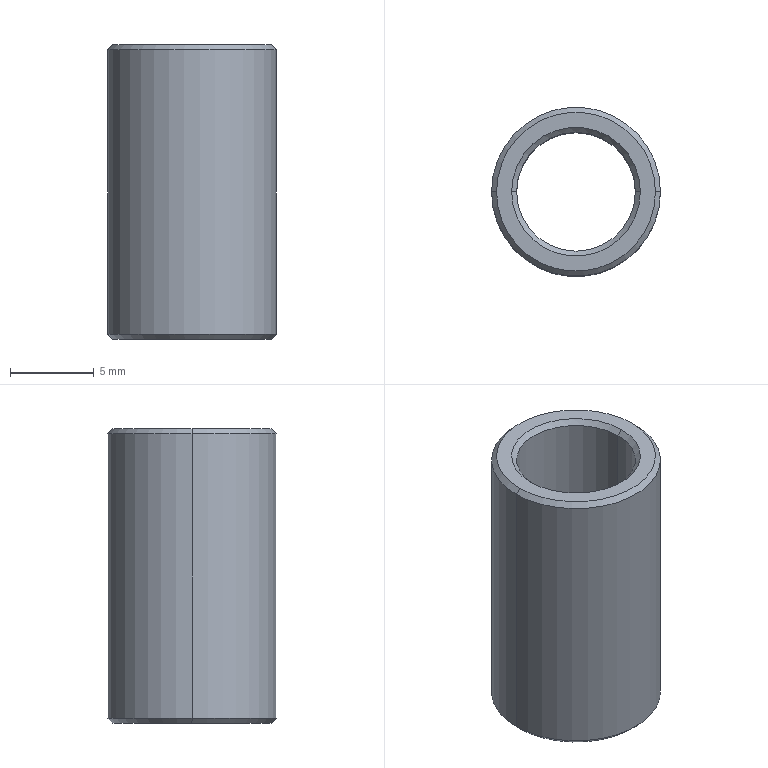Part | NX | features BREP 1 | 1 solid | 14 faces | box 10.1 x 10.1 x 17.6 mm | volume 708.404 mm3 | cone 8 | cylinder 4 | plane 2 | commonest cylinder face diameters 7.1 x2 10.1 x2
STEP:
#1=CARTESIAN_POINT('',(-5.05,0.,0.3));
#2=VERTEX_POINT('',#1);
#3=CARTESIAN_POINT('',(-4.75,0.,0.));
#4=VERTEX_POINT('',#3);
#5=CARTESIAN_POINT('',(-5.05,0.,0.3));
#6=DIRECTION('',(-0.7071,0.,0.7071));
#7=VECTOR('',#6,1000.);
#8=LINE('',#5,#7);
#9=EDGE_CURVE('',#2,#4,#8,.F.);
#10=ORIENTED_EDGE('',*,*,#9,.T.);
#11=CARTESIAN_POINT('',(4.75,0.,0.));
#12=VERTEX_POINT('',#11);
#13=CARTESIAN_POINT('',(0.,0.,0.));
#14=DIRECTION('',(0.,0.,-1.));
#15=DIRECTION('',(1.,0.,0.));
#16=AXIS2_PLACEMENT_3D('',#13,#14,#15);
#17=CIRCLE('',#16,4.75);
#18=EDGE_CURVE('',#12,#4,#17,.T.);
#19=ORIENTED_EDGE('',*,*,#18,.F.);
#20=CARTESIAN_POINT('',(5.05,0.,0.3));
#21=VERTEX_POINT('',#20);
#22=CARTESIAN_POINT('',(5.05,0.,0.3));
#23=DIRECTION('',(0.7071,0.,0.7071));
#24=VECTOR('',#23,1000.);
#25=LINE('',#22,#24);
#26=EDGE_CURVE('',#21,#12,#25,.F.);
#27=ORIENTED_EDGE('',*,*,#26,.F.);
#28=CARTESIAN_POINT('',(0.,0.,0.3));
#29=DIRECTION('',(0.,0.,1.));
#30=DIRECTION('',(1.,0.,0.));
#31=AXIS2_PLACEMENT_3D('',#28,#29,#30);
#32=CIRCLE('',#31,5.05);
#33=EDGE_CURVE('',#2,#21,#32,.T.);
#34=ORIENTED_EDGE('',*,*,#33,.F.);
#35=EDGE_LOOP('',(#10,#19,#27,#34));
#36=FACE_BOUND('',#35,.T.);
#37=CARTESIAN_POINT('',(0.,0.,0.3));
#38=DIRECTION('',(0.,0.,1.));
#39=DIRECTION('',(1.,0.,0.));
#40=AXIS2_PLACEMENT_3D('',#37,#38,#39);
#41=CONICAL_SURFACE('',#40,5.05,0.7854);
#42=ADVANCED_FACE('',(#36),#41,.T.);
#43=CARTESIAN_POINT('',(3.55,0.,0.3));
#44=VERTEX_POINT('',#43);
#45=CARTESIAN_POINT('',(3.85,0.,0.));
#46=VERTEX_POINT('',#45);
#47=CARTESIAN_POINT('',(3.85,0.,0.));
#48=DIRECTION('',(0.7071,0.,-0.7071));
#49=VECTOR('',#48,1000.);
#50=LINE('',#47,#49);
#51=EDGE_CURVE('',#44,#46,#50,.T.);
#52=ORIENTED_EDGE('',*,*,#51,.F.);
#53=CARTESIAN_POINT('',(-3.55,0.,0.3));
#54=VERTEX_POINT('',#53);
#55=CARTESIAN_POINT('',(0.,0.,0.3));
#56=DIRECTION('',(0.,0.,-1.));
#57=DIRECTION('',(1.,0.,0.));
#58=AXIS2_PLACEMENT_3D('',#55,#56,#57);
#59=CIRCLE('',#58,3.55);
#60=EDGE_CURVE('',#54,#44,#59,.T.);
#61=ORIENTED_EDGE('',*,*,#60,.F.);
#62=CARTESIAN_POINT('',(-3.85,0.,0.));
#63=VERTEX_POINT('',#62);
#64=CARTESIAN_POINT('',(-3.85,0.,0.));
#65=DIRECTION('',(-0.7071,0.,-0.7071));
#66=VECTOR('',#65,1000.);
#67=LINE('',#64,#66);
#68=EDGE_CURVE('',#54,#63,#67,.T.);
#69=ORIENTED_EDGE('',*,*,#68,.T.);
#70=CARTESIAN_POINT('',(0.,0.,0.));
#71=DIRECTION('',(0.,0.,1.));
#72=DIRECTION('',(1.,0.,0.));
#73=AXIS2_PLACEMENT_3D('',#70,#71,#72);
#74=CIRCLE('',#73,3.85);
#75=EDGE_CURVE('',#46,#63,#74,.T.);
#76=ORIENTED_EDGE('',*,*,#75,.F.);
#77=EDGE_LOOP('',(#52,#61,#69,#76));
#78=FACE_BOUND('',#77,.T.);
#79=CARTESIAN_POINT('',(0.,0.,0.));
#80=DIRECTION('',(0.,0.,-1.));
#81=DIRECTION('',(-1.,0.,0.));
#82=AXIS2_PLACEMENT_3D('',#79,#80,#81);
#83=CONICAL_SURFACE('',#82,3.85,0.7854);
#84=ADVANCED_FACE('',(#78),#83,.F.);
#85=CARTESIAN_POINT('',(4.75,0.,17.6));
#86=VERTEX_POINT('',#85);
#87=CARTESIAN_POINT('',(5.05,0.,17.3));
#88=VERTEX_POINT('',#87);
#89=CARTESIAN_POINT('',(4.75,0.,17.6));
#90=DIRECTION('',(0.7071,0.,-0.7071));
#91=VECTOR('',#90,1000.);
#92=LINE('',#89,#91);
#93=EDGE_CURVE('',#86,#88,#92,.T.);
#94=ORIENTED_EDGE('',*,*,#93,.F.);
#95=CARTESIAN_POINT('',(-4.75,0.,17.6));
#96=VERTEX_POINT('',#95);
#97=CARTESIAN_POINT('',(0.,0.,17.6));
#98=DIRECTION('',(0.,0.,1.));
#99=DIRECTION('',(1.,0.,0.));
#100=AXIS2_PLACEMENT_3D('',#97,#98,#99);
#101=CIRCLE('',#100,4.75);
#102=EDGE_CURVE('',#96,#86,#101,.T.);
#103=ORIENTED_EDGE('',*,*,#102,.F.);
#104=CARTESIAN_POINT('',(-5.05,0.,17.3));
#105=VERTEX_POINT('',#104);
#106=CARTESIAN_POINT('',(-4.75,0.,17.6));
#107=DIRECTION('',(-0.7071,0.,-0.7071));
#108=VECTOR('',#107,1000.);
#109=LINE('',#106,#108);
#110=EDGE_CURVE('',#96,#105,#109,.T.);
#111=ORIENTED_EDGE('',*,*,#110,.T.);
#112=CARTESIAN_POINT('',(0.,0.,17.3));
#113=DIRECTION('',(0.,0.,-1.));
#114=DIRECTION('',(1.,0.,0.));
#115=AXIS2_PLACEMENT_3D('',#112,#113,#114);
#116=CIRCLE('',#115,5.05);
#117=EDGE_CURVE('',#88,#105,#116,.T.);
#118=ORIENTED_EDGE('',*,*,#117,.F.);
#119=EDGE_LOOP('',(#94,#103,#111,#118));
#120=FACE_BOUND('',#119,.T.);
#121=CARTESIAN_POINT('',(0.,0.,17.6));
#122=DIRECTION('',(0.,0.,-1.));
#123=DIRECTION('',(-1.,0.,0.));
#124=AXIS2_PLACEMENT_3D('',#121,#122,#123);
#125=CONICAL_SURFACE('',#124,4.75,0.7854);
#126=ADVANCED_FACE('',(#120),#125,.T.);
#127=CARTESIAN_POINT('',(-3.85,0.,17.6));
#128=VERTEX_POINT('',#127);
#129=CARTESIAN_POINT('',(-3.55,0.,17.3));
#130=VERTEX_POINT('',#129);
#131=CARTESIAN_POINT('',(-3.55,0.,17.3));
#132=DIRECTION('',(-0.7071,0.,0.7071));
#133=VECTOR('',#132,1000.);
#134=LINE('',#131,#133);
#135=EDGE_CURVE('',#128,#130,#134,.F.);
#136=ORIENTED_EDGE('',*,*,#135,.T.);
#137=CARTESIAN_POINT('',(3.55,0.,17.3));
#138=VERTEX_POINT('',#137);
#139=CARTESIAN_POINT('',(0.,0.,17.3));
#140=DIRECTION('',(0.,0.,1.));
#141=DIRECTION('',(1.,0.,0.));
#142=AXIS2_PLACEMENT_3D('',#139,#140,#141);
#143=CIRCLE('',#142,3.55);
#144=EDGE_CURVE('',#138,#130,#143,.T.);
#145=ORIENTED_EDGE('',*,*,#144,.F.);
#146=CARTESIAN_POINT('',(3.85,0.,17.6));
#147=VERTEX_POINT('',#146);
#148=CARTESIAN_POINT('',(3.55,0.,17.3));
#149=DIRECTION('',(0.7071,0.,0.7071));
#150=VECTOR('',#149,1000.);
#151=LINE('',#148,#150);
#152=EDGE_CURVE('',#147,#138,#151,.F.);
#153=ORIENTED_EDGE('',*,*,#152,.F.);
#154=CARTESIAN_POINT('',(0.,0.,17.6));
#155=DIRECTION('',(0.,0.,-1.));
#156=DIRECTION('',(1.,0.,0.));
#157=AXIS2_PLACEMENT_3D('',#154,#155,#156);
#158=CIRCLE('',#157,3.85);
#159=EDGE_CURVE('',#128,#147,#158,.T.);
#160=ORIENTED_EDGE('',*,*,#159,.F.);
#161=EDGE_LOOP('',(#136,#145,#153,#160));
#162=FACE_BOUND('',#161,.T.);
#163=CARTESIAN_POINT('',(0.,0.,17.3));
#164=DIRECTION('',(0.,0.,1.));
#165=DIRECTION('',(1.,0.,0.));
#166=AXIS2_PLACEMENT_3D('',#163,#164,#165);
#167=CONICAL_SURFACE('',#166,3.55,0.7854);
#168=ADVANCED_FACE('',(#162),#167,.F.);
#169=CARTESIAN_POINT('',(3.55,0.,17.6));
#170=DIRECTION('',(0.,0.,-1.));
#171=VECTOR('',#170,1000.);
#172=LINE('',#169,#171);
#173=EDGE_CURVE('',#138,#44,#172,.T.);
#174=ORIENTED_EDGE('',*,*,#173,.F.);
#175=ORIENTED_EDGE('',*,*,#144,.T.);
#176=CARTESIAN_POINT('',(-3.55,0.,17.6));
#177=DIRECTION('',(0.,0.,-1.));
#178=VECTOR('',#177,1000.);
#179=LINE('',#176,#178);
#180=EDGE_CURVE('',#130,#54,#179,.T.);
#181=ORIENTED_EDGE('',*,*,#180,.T.);
#182=ORIENTED_EDGE('',*,*,#60,.T.);
#183=EDGE_LOOP('',(#174,#175,#181,#182));
#184=FACE_BOUND('',#183,.T.);
#185=CARTESIAN_POINT('',(0.,0.,17.6));
#186=DIRECTION('',(0.,0.,-1.));
#187=DIRECTION('',(-1.,0.,0.));
#188=AXIS2_PLACEMENT_3D('',#185,#186,#187);
#189=CYLINDRICAL_SURFACE('',#188,3.55);
#190=ADVANCED_FACE('',(#184),#189,.F.);
#191=CARTESIAN_POINT('',(5.05,0.,17.6));
#192=DIRECTION('',(0.,0.,-1.));
#193=VECTOR('',#192,1000.);
#194=LINE('',#191,#193);
#195=EDGE_CURVE('',#88,#21,#194,.T.);
#196=ORIENTED_EDGE('',*,*,#195,.F.);
#197=ORIENTED_EDGE('',*,*,#117,.T.);
#198=CARTESIAN_POINT('',(-5.05,0.,17.6));
#199=DIRECTION('',(0.,0.,-1.));
#200=VECTOR('',#199,1000.);
#201=LINE('',#198,#200);
#202=EDGE_CURVE('',#105,#2,#201,.T.);
#203=ORIENTED_EDGE('',*,*,#202,.T.);
#204=ORIENTED_EDGE('',*,*,#33,.T.);
#205=EDGE_LOOP('',(#196,#197,#203,#204));
#206=FACE_BOUND('',#205,.T.);
#207=CARTESIAN_POINT('',(0.,0.,17.6));
#208=DIRECTION('',(0.,0.,-1.));
#209=DIRECTION('',(-1.,0.,0.));
#210=AXIS2_PLACEMENT_3D('',#207,#208,#209);
#211=CYLINDRICAL_SURFACE('',#210,5.05);
#212=ADVANCED_FACE('',(#206),#211,.T.);
#213=ORIENTED_EDGE('',*,*,#18,.T.);
#214=CARTESIAN_POINT('',(0.,0.,0.));
#215=DIRECTION('',(0.,0.,-1.));
#216=DIRECTION('',(1.,0.,0.));
#217=AXIS2_PLACEMENT_3D('',#214,#215,#216);
#218=CIRCLE('',#217,4.75);
#219=EDGE_CURVE('',#4,#12,#218,.T.);
#220=ORIENTED_EDGE('',*,*,#219,.T.);
#221=EDGE_LOOP('',(#213,#220));
#222=FACE_BOUND('',#221,.T.);
#223=CARTESIAN_POINT('',(0.,0.,0.));
#224=DIRECTION('',(0.,0.,1.));
#225=DIRECTION('',(1.,0.,0.));
#226=AXIS2_PLACEMENT_3D('',#223,#224,#225);
#227=CIRCLE('',#226,3.85);
#228=EDGE_CURVE('',#63,#46,#227,.T.);
#229=ORIENTED_EDGE('',*,*,#228,.T.);
#230=ORIENTED_EDGE('',*,*,#75,.T.);
#231=EDGE_LOOP('',(#229,#230));
#232=FACE_BOUND('',#231,.T.);
#233=CARTESIAN_POINT('',(0.,0.,0.));
#234=DIRECTION('',(0.,0.,1.));
#235=DIRECTION('',(1.,0.,0.));
#236=AXIS2_PLACEMENT_3D('',#233,#234,#235);
#237=PLANE('',#236);
#238=ADVANCED_FACE('',(#222,#232),#237,.F.);
#239=ORIENTED_EDGE('',*,*,#102,.T.);
#240=CARTESIAN_POINT('',(0.,0.,17.6));
#241=DIRECTION('',(0.,0.,1.));
#242=DIRECTION('',(1.,0.,0.));
#243=AXIS2_PLACEMENT_3D('',#240,#241,#242);
#244=CIRCLE('',#243,4.75);
#245=EDGE_CURVE('',#86,#96,#244,.T.);
#246=ORIENTED_EDGE('',*,*,#245,.T.);
#247=EDGE_LOOP('',(#239,#246));
#248=FACE_BOUND('',#247,.T.);
#249=CARTESIAN_POINT('',(0.,0.,17.6));
#250=DIRECTION('',(0.,0.,-1.));
#251=DIRECTION('',(1.,0.,0.));
#252=AXIS2_PLACEMENT_3D('',#249,#250,#251);
#253=CIRCLE('',#252,3.85);
#254=EDGE_CURVE('',#147,#128,#253,.T.);
#255=ORIENTED_EDGE('',*,*,#254,.T.);
#256=ORIENTED_EDGE('',*,*,#159,.T.);
#257=EDGE_LOOP('',(#255,#256));
#258=FACE_BOUND('',#257,.T.);
#259=CARTESIAN_POINT('',(0.,0.,17.6));
#260=DIRECTION('',(0.,0.,1.));
#261=DIRECTION('',(1.,0.,0.));
#262=AXIS2_PLACEMENT_3D('',#259,#260,#261);
#263=PLANE('',#262);
#264=ADVANCED_FACE('',(#248,#258),#263,.T.);
#265=CARTESIAN_POINT('',(0.,0.,17.3));
#266=DIRECTION('',(0.,0.,-1.));
#267=DIRECTION('',(1.,0.,0.));
#268=AXIS2_PLACEMENT_3D('',#265,#266,#267);
#269=CIRCLE('',#268,5.05);
#270=EDGE_CURVE('',#105,#88,#269,.T.);
#271=ORIENTED_EDGE('',*,*,#270,.T.);
#272=ORIENTED_EDGE('',*,*,#195,.T.);
#273=CARTESIAN_POINT('',(0.,0.,0.3));
#274=DIRECTION('',(0.,0.,1.));
#275=DIRECTION('',(1.,0.,0.));
#276=AXIS2_PLACEMENT_3D('',#273,#274,#275);
#277=CIRCLE('',#276,5.05);
#278=EDGE_CURVE('',#21,#2,#277,.T.);
#279=ORIENTED_EDGE('',*,*,#278,.T.);
#280=ORIENTED_EDGE('',*,*,#202,.F.);
#281=EDGE_LOOP('',(#271,#272,#279,#280));
#282=FACE_BOUND('',#281,.T.);
#283=CARTESIAN_POINT('',(0.,0.,17.6));
#284=DIRECTION('',(0.,0.,-1.));
#285=DIRECTION('',(-1.,0.,0.));
#286=AXIS2_PLACEMENT_3D('',#283,#284,#285);
#287=CYLINDRICAL_SURFACE('',#286,5.05);
#288=ADVANCED_FACE('',(#282),#287,.T.);
#289=CARTESIAN_POINT('',(0.,0.,17.3));
#290=DIRECTION('',(0.,0.,1.));
#291=DIRECTION('',(1.,0.,0.));
#292=AXIS2_PLACEMENT_3D('',#289,#290,#291);
#293=CIRCLE('',#292,3.55);
#294=EDGE_CURVE('',#130,#138,#293,.T.);
#295=ORIENTED_EDGE('',*,*,#294,.T.);
#296=ORIENTED_EDGE('',*,*,#173,.T.);
#297=CARTESIAN_POINT('',(0.,0.,0.3));
#298=DIRECTION('',(0.,0.,-1.));
#299=DIRECTION('',(1.,0.,0.));
#300=AXIS2_PLACEMENT_3D('',#297,#298,#299);
#301=CIRCLE('',#300,3.55);
#302=EDGE_CURVE('',#44,#54,#301,.T.);
#303=ORIENTED_EDGE('',*,*,#302,.T.);
#304=ORIENTED_EDGE('',*,*,#180,.F.);
#305=EDGE_LOOP('',(#295,#296,#303,#304));
#306=FACE_BOUND('',#305,.T.);
#307=CARTESIAN_POINT('',(0.,0.,17.6));
#308=DIRECTION('',(0.,0.,-1.));
#309=DIRECTION('',(-1.,0.,0.));
#310=AXIS2_PLACEMENT_3D('',#307,#308,#309);
#311=CYLINDRICAL_SURFACE('',#310,3.55);
#312=ADVANCED_FACE('',(#306),#311,.F.);
#313=ORIENTED_EDGE('',*,*,#294,.F.);
#314=ORIENTED_EDGE('',*,*,#135,.F.);
#315=ORIENTED_EDGE('',*,*,#254,.F.);
#316=ORIENTED_EDGE('',*,*,#152,.T.);
#317=EDGE_LOOP('',(#313,#314,#315,#316));
#318=FACE_BOUND('',#317,.T.);
#319=CARTESIAN_POINT('',(0.,0.,17.3));
#320=DIRECTION('',(0.,0.,1.));
#321=DIRECTION('',(1.,0.,0.));
#322=AXIS2_PLACEMENT_3D('',#319,#320,#321);
#323=CONICAL_SURFACE('',#322,3.55,0.7854);
#324=ADVANCED_FACE('',(#318),#323,.F.);
#325=ORIENTED_EDGE('',*,*,#245,.F.);
#326=ORIENTED_EDGE('',*,*,#93,.T.);
#327=ORIENTED_EDGE('',*,*,#270,.F.);
#328=ORIENTED_EDGE('',*,*,#110,.F.);
#329=EDGE_LOOP('',(#325,#326,#327,#328));
#330=FACE_BOUND('',#329,.T.);
#331=CARTESIAN_POINT('',(0.,0.,17.6));
#332=DIRECTION('',(0.,0.,-1.));
#333=DIRECTION('',(-1.,0.,0.));
#334=AXIS2_PLACEMENT_3D('',#331,#332,#333);
#335=CONICAL_SURFACE('',#334,4.75,0.7854);
#336=ADVANCED_FACE('',(#330),#335,.T.);
#337=ORIENTED_EDGE('',*,*,#302,.F.);
#338=ORIENTED_EDGE('',*,*,#51,.T.);
#339=ORIENTED_EDGE('',*,*,#228,.F.);
#340=ORIENTED_EDGE('',*,*,#68,.F.);
#341=EDGE_LOOP('',(#337,#338,#339,#340));
#342=FACE_BOUND('',#341,.T.);
#343=CARTESIAN_POINT('',(0.,0.,0.));
#344=DIRECTION('',(0.,0.,-1.));
#345=DIRECTION('',(-1.,0.,0.));
#346=AXIS2_PLACEMENT_3D('',#343,#344,#345);
#347=CONICAL_SURFACE('',#346,3.85,0.7854);
#348=ADVANCED_FACE('',(#342),#347,.F.);
#349=ORIENTED_EDGE('',*,*,#219,.F.);
#350=ORIENTED_EDGE('',*,*,#9,.F.);
#351=ORIENTED_EDGE('',*,*,#278,.F.);
#352=ORIENTED_EDGE('',*,*,#26,.T.);
#353=EDGE_LOOP('',(#349,#350,#351,#352));
#354=FACE_BOUND('',#353,.T.);
#355=CARTESIAN_POINT('',(0.,0.,0.3));
#356=DIRECTION('',(0.,0.,1.));
#357=DIRECTION('',(1.,0.,0.));
#358=AXIS2_PLACEMENT_3D('',#355,#356,#357);
#359=CONICAL_SURFACE('',#358,5.05,0.7854);
#360=ADVANCED_FACE('',(#354),#359,.T.);
#361=CLOSED_SHELL('',(#42,#84,#126,#168,#190,#212,#238,#264,#288,#312,#324,#336,#348,#360));
#362=MANIFOLD_SOLID_BREP('',#361);
#363=(LENGTH_UNIT()NAMED_UNIT(*)SI_UNIT(.MILLI.,.METRE.));
#364=UNCERTAINTY_MEASURE_WITH_UNIT(LENGTH_MEASURE(0.00001),#363,'','');
#365=(NAMED_UNIT(*)PLANE_ANGLE_UNIT()SI_UNIT($,.RADIAN.));
#366=(NAMED_UNIT(*)SI_UNIT($,.STERADIAN.)SOLID_ANGLE_UNIT());
#367=(GEOMETRIC_REPRESENTATION_CONTEXT(3)GLOBAL_UNCERTAINTY_ASSIGNED_CONTEXT((#364))GLOBAL_UNIT_ASSIGNED_CONTEXT((#363,#365,#366))REPRESENTATION_CONTEXT('',''));
#368=ADVANCED_BREP_SHAPE_REPRESENTATION('',(#362),#367);